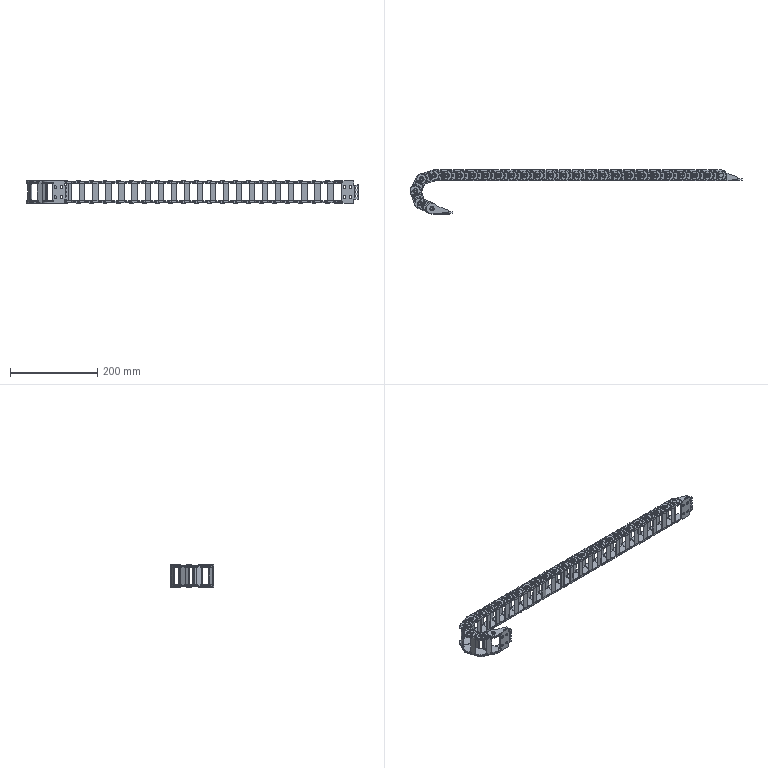Part | STEP file | C-MPU20-40-38-26-S20-9 | 28 solids | 6316 faces | volume 259932 mm3 | plane 4172 | cylinder 1032 | spline 1008 | cone 104 | commonest cylinder face diameters 2 x260 25 x212 1.6 x208 10 x108 2.4 x104 12 x52